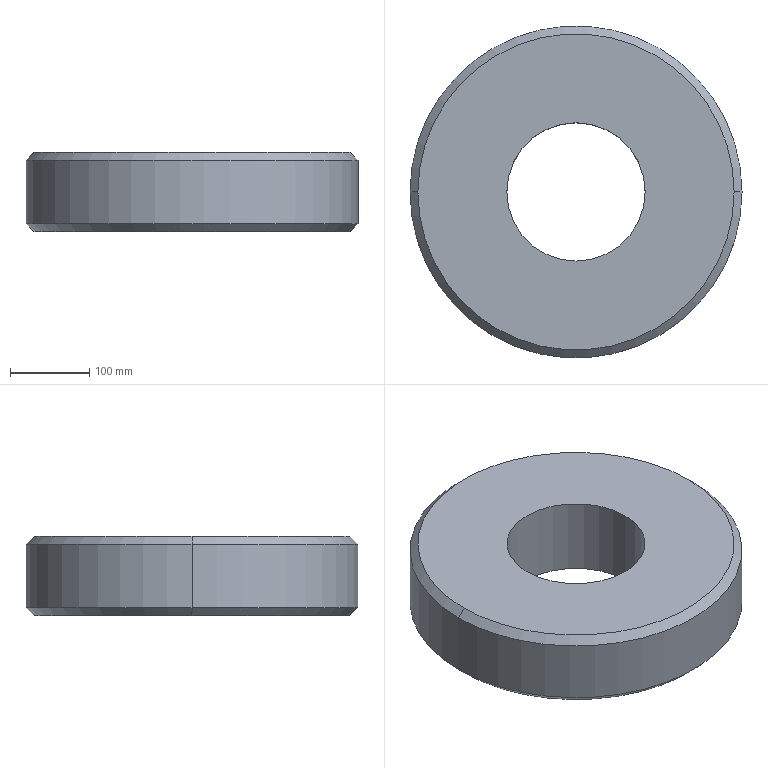Part | SolidWorks | features Chamfer 1, Extrusion 1 | 1 solid | 10 faces | box 420 x 420 x 100 mm | volume 11319289 mm3 | cone 4 | cylinder 4 | plane 2 | commonest cylinder face diameters 175 x2 420 x2
STEP:
#1=CARTESIAN_POINT('',(200.,0.,100.));
#2=VERTEX_POINT('',#1);
#3=CARTESIAN_POINT('',(-200.,0.,100.));
#4=VERTEX_POINT('',#3);
#5=CARTESIAN_POINT('',(0.,0.,100.));
#6=DIRECTION('',(0.,0.,1.));
#7=DIRECTION('',(1.,0.,0.));
#8=AXIS2_PLACEMENT_3D('',#5,#6,#7);
#9=CIRCLE('',#8,200.);
#10=EDGE_CURVE('',#2,#4,#9,.T.);
#11=ORIENTED_EDGE('',*,*,#10,.F.);
#12=CARTESIAN_POINT('',(210.,0.,90.));
#13=VERTEX_POINT('',#12);
#14=CARTESIAN_POINT('',(200.,0.,100.));
#15=DIRECTION('',(0.7071,0.,-0.7071));
#16=VECTOR('',#15,1000.);
#17=LINE('',#14,#16);
#18=EDGE_CURVE('',#2,#13,#17,.T.);
#19=ORIENTED_EDGE('',*,*,#18,.T.);
#20=CARTESIAN_POINT('',(-210.,0.,90.));
#21=VERTEX_POINT('',#20);
#22=CARTESIAN_POINT('',(0.,0.,90.));
#23=DIRECTION('',(0.,0.,-1.));
#24=DIRECTION('',(1.,0.,0.));
#25=AXIS2_PLACEMENT_3D('',#22,#23,#24);
#26=CIRCLE('',#25,210.);
#27=EDGE_CURVE('',#21,#13,#26,.T.);
#28=ORIENTED_EDGE('',*,*,#27,.F.);
#29=CARTESIAN_POINT('',(-200.,0.,100.));
#30=DIRECTION('',(-0.7071,0.,-0.7071));
#31=VECTOR('',#30,1000.);
#32=LINE('',#29,#31);
#33=EDGE_CURVE('',#4,#21,#32,.T.);
#34=ORIENTED_EDGE('',*,*,#33,.F.);
#35=EDGE_LOOP('',(#11,#19,#28,#34));
#36=FACE_OUTER_BOUND('',#35,.T.);
#37=CARTESIAN_POINT('',(0.,0.,100.));
#38=DIRECTION('',(0.,0.,-1.));
#39=DIRECTION('',(-1.,0.,0.));
#40=AXIS2_PLACEMENT_3D('',#37,#38,#39);
#41=CONICAL_SURFACE('',#40,200.,0.7854);
#42=ADVANCED_FACE('',(#36),#41,.T.);
#43=CARTESIAN_POINT('',(-200.,0.,0.));
#44=VERTEX_POINT('',#43);
#45=CARTESIAN_POINT('',(200.,0.,0.));
#46=VERTEX_POINT('',#45);
#47=CARTESIAN_POINT('',(0.,0.,0.));
#48=DIRECTION('',(0.,0.,-1.));
#49=DIRECTION('',(1.,0.,0.));
#50=AXIS2_PLACEMENT_3D('',#47,#48,#49);
#51=CIRCLE('',#50,200.);
#52=EDGE_CURVE('',#44,#46,#51,.T.);
#53=ORIENTED_EDGE('',*,*,#52,.F.);
#54=CARTESIAN_POINT('',(-210.,0.,10.));
#55=VERTEX_POINT('',#54);
#56=CARTESIAN_POINT('',(-210.,0.,10.));
#57=DIRECTION('',(-0.7071,0.,0.7071));
#58=VECTOR('',#57,1000.);
#59=LINE('',#56,#58);
#60=EDGE_CURVE('',#44,#55,#59,.T.);
#61=ORIENTED_EDGE('',*,*,#60,.T.);
#62=CARTESIAN_POINT('',(210.,0.,10.));
#63=VERTEX_POINT('',#62);
#64=CARTESIAN_POINT('',(0.,0.,10.));
#65=DIRECTION('',(0.,0.,1.));
#66=DIRECTION('',(1.,0.,0.));
#67=AXIS2_PLACEMENT_3D('',#64,#65,#66);
#68=CIRCLE('',#67,210.);
#69=EDGE_CURVE('',#63,#55,#68,.T.);
#70=ORIENTED_EDGE('',*,*,#69,.F.);
#71=CARTESIAN_POINT('',(210.,0.,10.));
#72=DIRECTION('',(0.7071,0.,0.7071));
#73=VECTOR('',#72,1000.);
#74=LINE('',#71,#73);
#75=EDGE_CURVE('',#46,#63,#74,.T.);
#76=ORIENTED_EDGE('',*,*,#75,.F.);
#77=EDGE_LOOP('',(#53,#61,#70,#76));
#78=FACE_OUTER_BOUND('',#77,.T.);
#79=CARTESIAN_POINT('',(0.,0.,10.));
#80=DIRECTION('',(0.,0.,1.));
#81=DIRECTION('',(1.,0.,0.));
#82=AXIS2_PLACEMENT_3D('',#79,#80,#81);
#83=CONICAL_SURFACE('',#82,210.,0.7854);
#84=ADVANCED_FACE('',(#78),#83,.T.);
#85=CARTESIAN_POINT('',(-87.5,0.,100.));
#86=VERTEX_POINT('',#85);
#87=CARTESIAN_POINT('',(87.5,0.,100.));
#88=VERTEX_POINT('',#87);
#89=CARTESIAN_POINT('',(0.,0.,100.));
#90=DIRECTION('',(0.,0.,1.));
#91=DIRECTION('',(1.,0.,0.));
#92=AXIS2_PLACEMENT_3D('',#89,#90,#91);
#93=CIRCLE('',#92,87.5);
#94=EDGE_CURVE('',#86,#88,#93,.T.);
#95=ORIENTED_EDGE('',*,*,#94,.T.);
#96=CARTESIAN_POINT('',(87.5,0.,0.));
#97=VERTEX_POINT('',#96);
#98=CARTESIAN_POINT('',(87.5,0.,100.));
#99=DIRECTION('',(0.,0.,-1.));
#100=VECTOR('',#99,1000.);
#101=LINE('',#98,#100);
#102=EDGE_CURVE('',#88,#97,#101,.T.);
#103=ORIENTED_EDGE('',*,*,#102,.T.);
#104=CARTESIAN_POINT('',(-87.5,0.,0.));
#105=VERTEX_POINT('',#104);
#106=CARTESIAN_POINT('',(0.,0.,0.));
#107=DIRECTION('',(0.,0.,1.));
#108=DIRECTION('',(1.,0.,0.));
#109=AXIS2_PLACEMENT_3D('',#106,#107,#108);
#110=CIRCLE('',#109,87.5);
#111=EDGE_CURVE('',#105,#97,#110,.T.);
#112=ORIENTED_EDGE('',*,*,#111,.F.);
#113=CARTESIAN_POINT('',(-87.5,0.,100.));
#114=DIRECTION('',(0.,0.,-1.));
#115=VECTOR('',#114,1000.);
#116=LINE('',#113,#115);
#117=EDGE_CURVE('',#86,#105,#116,.T.);
#118=ORIENTED_EDGE('',*,*,#117,.F.);
#119=EDGE_LOOP('',(#95,#103,#112,#118));
#120=FACE_OUTER_BOUND('',#119,.T.);
#121=CARTESIAN_POINT('',(0.,0.,100.));
#122=DIRECTION('',(0.,0.,-1.));
#123=DIRECTION('',(-1.,0.,0.));
#124=AXIS2_PLACEMENT_3D('',#121,#122,#123);
#125=CYLINDRICAL_SURFACE('',#124,87.5);
#126=ADVANCED_FACE('',(#120),#125,.F.);
#127=ORIENTED_EDGE('',*,*,#27,.T.);
#128=CARTESIAN_POINT('',(210.,0.,100.));
#129=DIRECTION('',(0.,0.,-1.));
#130=VECTOR('',#129,1000.);
#131=LINE('',#128,#130);
#132=EDGE_CURVE('',#13,#63,#131,.T.);
#133=ORIENTED_EDGE('',*,*,#132,.T.);
#134=ORIENTED_EDGE('',*,*,#69,.T.);
#135=CARTESIAN_POINT('',(-210.,0.,100.));
#136=DIRECTION('',(0.,0.,-1.));
#137=VECTOR('',#136,1000.);
#138=LINE('',#135,#137);
#139=EDGE_CURVE('',#21,#55,#138,.T.);
#140=ORIENTED_EDGE('',*,*,#139,.F.);
#141=EDGE_LOOP('',(#127,#133,#134,#140));
#142=FACE_OUTER_BOUND('',#141,.T.);
#143=CARTESIAN_POINT('',(0.,0.,100.));
#144=DIRECTION('',(0.,0.,-1.));
#145=DIRECTION('',(-1.,0.,0.));
#146=AXIS2_PLACEMENT_3D('',#143,#144,#145);
#147=CYLINDRICAL_SURFACE('',#146,210.);
#148=ADVANCED_FACE('',(#142),#147,.T.);
#149=CARTESIAN_POINT('',(0.,0.,100.));
#150=DIRECTION('',(0.,0.,1.));
#151=DIRECTION('',(1.,0.,0.));
#152=AXIS2_PLACEMENT_3D('',#149,#150,#151);
#153=CIRCLE('',#152,200.);
#154=EDGE_CURVE('',#4,#2,#153,.T.);
#155=ORIENTED_EDGE('',*,*,#154,.T.);
#156=ORIENTED_EDGE('',*,*,#10,.T.);
#157=EDGE_LOOP('',(#155,#156));
#158=FACE_OUTER_BOUND('',#157,.T.);
#159=ORIENTED_EDGE('',*,*,#94,.F.);
#160=CARTESIAN_POINT('',(0.,0.,100.));
#161=DIRECTION('',(0.,0.,1.));
#162=DIRECTION('',(1.,0.,0.));
#163=AXIS2_PLACEMENT_3D('',#160,#161,#162);
#164=CIRCLE('',#163,87.5);
#165=EDGE_CURVE('',#88,#86,#164,.T.);
#166=ORIENTED_EDGE('',*,*,#165,.F.);
#167=EDGE_LOOP('',(#159,#166));
#168=FACE_BOUND('',#167,.T.);
#169=CARTESIAN_POINT('',(0.,0.,100.));
#170=DIRECTION('',(0.,0.,1.));
#171=DIRECTION('',(1.,0.,0.));
#172=AXIS2_PLACEMENT_3D('',#169,#170,#171);
#173=PLANE('',#172);
#174=ADVANCED_FACE('',(#158,#168),#173,.T.);
#175=CARTESIAN_POINT('',(0.,0.,0.));
#176=DIRECTION('',(0.,0.,-1.));
#177=DIRECTION('',(1.,0.,0.));
#178=AXIS2_PLACEMENT_3D('',#175,#176,#177);
#179=CIRCLE('',#178,200.);
#180=EDGE_CURVE('',#46,#44,#179,.T.);
#181=ORIENTED_EDGE('',*,*,#180,.T.);
#182=ORIENTED_EDGE('',*,*,#52,.T.);
#183=EDGE_LOOP('',(#181,#182));
#184=FACE_OUTER_BOUND('',#183,.T.);
#185=ORIENTED_EDGE('',*,*,#111,.T.);
#186=CARTESIAN_POINT('',(0.,0.,0.));
#187=DIRECTION('',(0.,0.,1.));
#188=DIRECTION('',(1.,0.,0.));
#189=AXIS2_PLACEMENT_3D('',#186,#187,#188);
#190=CIRCLE('',#189,87.5);
#191=EDGE_CURVE('',#97,#105,#190,.T.);
#192=ORIENTED_EDGE('',*,*,#191,.T.);
#193=EDGE_LOOP('',(#185,#192));
#194=FACE_BOUND('',#193,.T.);
#195=CARTESIAN_POINT('',(0.,0.,0.));
#196=DIRECTION('',(0.,0.,1.));
#197=DIRECTION('',(1.,0.,0.));
#198=AXIS2_PLACEMENT_3D('',#195,#196,#197);
#199=PLANE('',#198);
#200=ADVANCED_FACE('',(#184,#194),#199,.F.);
#201=ORIENTED_EDGE('',*,*,#132,.F.);
#202=CARTESIAN_POINT('',(0.,0.,90.));
#203=DIRECTION('',(0.,0.,-1.));
#204=DIRECTION('',(1.,0.,0.));
#205=AXIS2_PLACEMENT_3D('',#202,#203,#204);
#206=CIRCLE('',#205,210.);
#207=EDGE_CURVE('',#13,#21,#206,.T.);
#208=ORIENTED_EDGE('',*,*,#207,.T.);
#209=ORIENTED_EDGE('',*,*,#139,.T.);
#210=CARTESIAN_POINT('',(0.,0.,10.));
#211=DIRECTION('',(0.,0.,1.));
#212=DIRECTION('',(1.,0.,0.));
#213=AXIS2_PLACEMENT_3D('',#210,#211,#212);
#214=CIRCLE('',#213,210.);
#215=EDGE_CURVE('',#55,#63,#214,.T.);
#216=ORIENTED_EDGE('',*,*,#215,.T.);
#217=EDGE_LOOP('',(#201,#208,#209,#216));
#218=FACE_OUTER_BOUND('',#217,.T.);
#219=CARTESIAN_POINT('',(0.,0.,100.));
#220=DIRECTION('',(0.,0.,-1.));
#221=DIRECTION('',(-1.,0.,0.));
#222=AXIS2_PLACEMENT_3D('',#219,#220,#221);
#223=CYLINDRICAL_SURFACE('',#222,210.);
#224=ADVANCED_FACE('',(#218),#223,.T.);
#225=ORIENTED_EDGE('',*,*,#102,.F.);
#226=ORIENTED_EDGE('',*,*,#165,.T.);
#227=ORIENTED_EDGE('',*,*,#117,.T.);
#228=ORIENTED_EDGE('',*,*,#191,.F.);
#229=EDGE_LOOP('',(#225,#226,#227,#228));
#230=FACE_OUTER_BOUND('',#229,.T.);
#231=CARTESIAN_POINT('',(0.,0.,100.));
#232=DIRECTION('',(0.,0.,-1.));
#233=DIRECTION('',(-1.,0.,0.));
#234=AXIS2_PLACEMENT_3D('',#231,#232,#233);
#235=CYLINDRICAL_SURFACE('',#234,87.5);
#236=ADVANCED_FACE('',(#230),#235,.F.);
#237=ORIENTED_EDGE('',*,*,#60,.F.);
#238=ORIENTED_EDGE('',*,*,#180,.F.);
#239=ORIENTED_EDGE('',*,*,#75,.T.);
#240=ORIENTED_EDGE('',*,*,#215,.F.);
#241=EDGE_LOOP('',(#237,#238,#239,#240));
#242=FACE_OUTER_BOUND('',#241,.T.);
#243=CARTESIAN_POINT('',(0.,0.,10.));
#244=DIRECTION('',(0.,0.,1.));
#245=DIRECTION('',(1.,0.,0.));
#246=AXIS2_PLACEMENT_3D('',#243,#244,#245);
#247=CONICAL_SURFACE('',#246,210.,0.7854);
#248=ADVANCED_FACE('',(#242),#247,.T.);
#249=ORIENTED_EDGE('',*,*,#18,.F.);
#250=ORIENTED_EDGE('',*,*,#154,.F.);
#251=ORIENTED_EDGE('',*,*,#33,.T.);
#252=ORIENTED_EDGE('',*,*,#207,.F.);
#253=EDGE_LOOP('',(#249,#250,#251,#252));
#254=FACE_OUTER_BOUND('',#253,.T.);
#255=CARTESIAN_POINT('',(0.,0.,100.));
#256=DIRECTION('',(0.,0.,-1.));
#257=DIRECTION('',(-1.,0.,0.));
#258=AXIS2_PLACEMENT_3D('',#255,#256,#257);
#259=CONICAL_SURFACE('',#258,200.,0.7854);
#260=ADVANCED_FACE('',(#254),#259,.T.);
#261=CLOSED_SHELL('',(#42,#84,#126,#148,#174,#200,#224,#236,#248,#260));
#262=MANIFOLD_SOLID_BREP('',#261);
#263=CARTESIAN_POINT('',(0.,0.,0.));
#264=DIRECTION('',(0.,0.,1.));
#265=DIRECTION('',(1.,0.,0.));
#266=AXIS2_PLACEMENT_3D('',#263,#264,#265);
#267=(LENGTH_UNIT()NAMED_UNIT(*)SI_UNIT(.MILLI.,.METRE.));
#268=UNCERTAINTY_MEASURE_WITH_UNIT(LENGTH_MEASURE(0.00001),#267,'','');
#269=(NAMED_UNIT(*)PLANE_ANGLE_UNIT()SI_UNIT($,.RADIAN.));
#270=(NAMED_UNIT(*)SI_UNIT($,.STERADIAN.)SOLID_ANGLE_UNIT());
#271=(GEOMETRIC_REPRESENTATION_CONTEXT(3)GLOBAL_UNCERTAINTY_ASSIGNED_CONTEXT((#268))GLOBAL_UNIT_ASSIGNED_CONTEXT((#267,#269,#270))REPRESENTATION_CONTEXT('',''));
#272=ADVANCED_BREP_SHAPE_REPRESENTATION('',(#262,#266),#271);